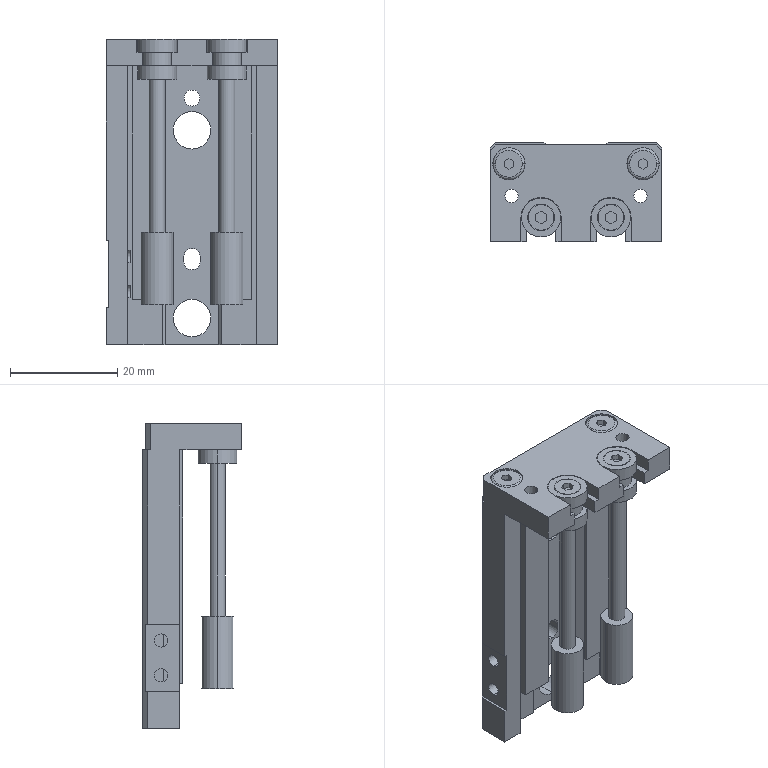Part | STEP file | QA-HI_MDX6x20-SG2BM2(0)_Ro | 1 solid | 173 faces | box 32 x 18.5 x 57 mm | volume 12589 mm3 | plane 112 | cylinder 57 | spline 4 | commonest cylinder face diameters 2.459 x16 3 x9 6 x8 7.3 x8 4.8 x4 5 x4